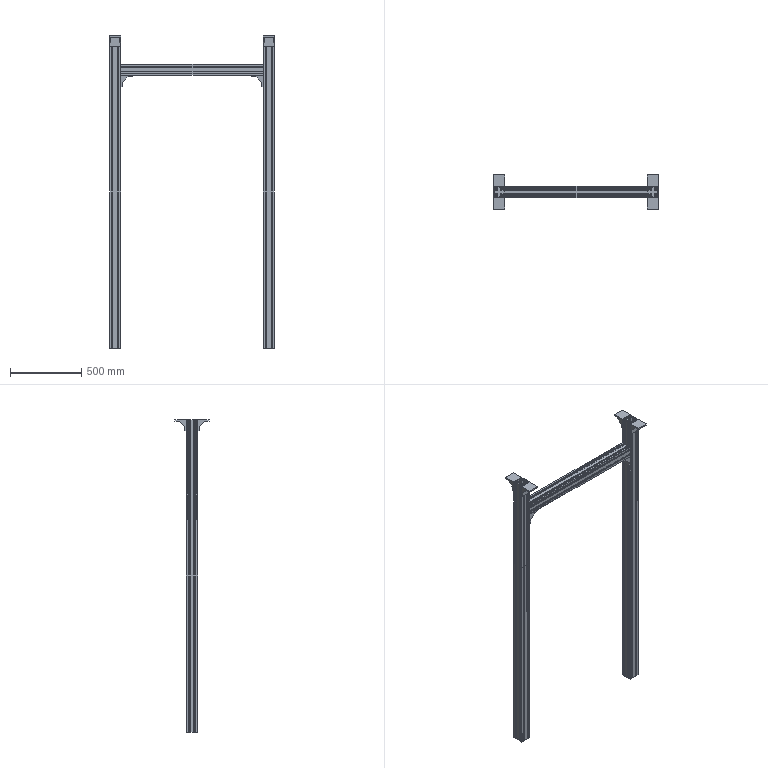Part | NX | features BREP 3 | 9 solids | 480 faces | box 1160 x 240 x 2200 mm | volume 22175197 mm3 | plane 432 | cylinder 48 | commonest cylinder face diameters 6.8 x48